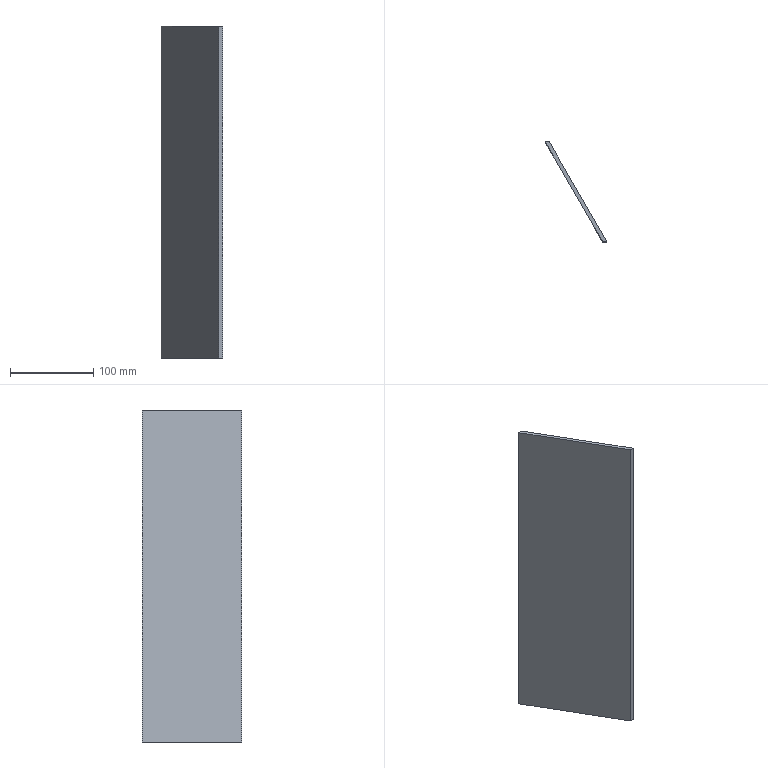Part | SolidWorks | features Extrusion 1 | 1 solid | 6 faces | box 74.282 x 120 x 400 mm | volume 240000 mm3 | plane 6
STEP:
#1=CARTESIAN_POINT('',(0.,0.,0.));
#2=VERTEX_POINT('',#1);
#3=CARTESIAN_POINT('',(69.282,-120.,0.));
#4=VERTEX_POINT('',#3);
#5=CARTESIAN_POINT('',(69.282,-120.,0.));
#6=DIRECTION('',(0.5,-0.866,0.));
#7=VECTOR('',#6,1000.);
#8=LINE('',#5,#7);
#9=EDGE_CURVE('',#2,#4,#8,.T.);
#10=ORIENTED_EDGE('',*,*,#9,.T.);
#11=CARTESIAN_POINT('',(69.282,-120.,400.));
#12=VERTEX_POINT('',#11);
#13=CARTESIAN_POINT('',(69.282,-120.,400.));
#14=DIRECTION('',(0.,0.,-1.));
#15=VECTOR('',#14,1000.);
#16=LINE('',#13,#15);
#17=EDGE_CURVE('',#12,#4,#16,.T.);
#18=ORIENTED_EDGE('',*,*,#17,.F.);
#19=CARTESIAN_POINT('',(0.,0.,400.));
#20=VERTEX_POINT('',#19);
#21=CARTESIAN_POINT('',(69.282,-120.,400.));
#22=DIRECTION('',(0.5,-0.866,0.));
#23=VECTOR('',#22,1000.);
#24=LINE('',#21,#23);
#25=EDGE_CURVE('',#20,#12,#24,.T.);
#26=ORIENTED_EDGE('',*,*,#25,.F.);
#27=CARTESIAN_POINT('',(0.,0.,400.));
#28=DIRECTION('',(0.,0.,-1.));
#29=VECTOR('',#28,1000.);
#30=LINE('',#27,#29);
#31=EDGE_CURVE('',#20,#2,#30,.T.);
#32=ORIENTED_EDGE('',*,*,#31,.T.);
#33=EDGE_LOOP('',(#10,#18,#26,#32));
#34=FACE_OUTER_BOUND('',#33,.T.);
#35=CARTESIAN_POINT('',(69.282,-120.,400.));
#36=DIRECTION('',(0.866,0.5,0.));
#37=DIRECTION('',(-0.5,0.866,0.));
#38=AXIS2_PLACEMENT_3D('',#35,#36,#37);
#39=PLANE('',#38);
#40=ADVANCED_FACE('',(#34),#39,.F.);
#41=CARTESIAN_POINT('',(74.282,-120.,0.));
#42=VERTEX_POINT('',#41);
#43=CARTESIAN_POINT('',(74.282,-120.,0.));
#44=DIRECTION('',(1.,0.,0.));
#45=VECTOR('',#44,1000.);
#46=LINE('',#43,#45);
#47=EDGE_CURVE('',#4,#42,#46,.T.);
#48=ORIENTED_EDGE('',*,*,#47,.T.);
#49=CARTESIAN_POINT('',(74.282,-120.,400.));
#50=VERTEX_POINT('',#49);
#51=CARTESIAN_POINT('',(74.282,-120.,400.));
#52=DIRECTION('',(0.,0.,-1.));
#53=VECTOR('',#52,1000.);
#54=LINE('',#51,#53);
#55=EDGE_CURVE('',#50,#42,#54,.T.);
#56=ORIENTED_EDGE('',*,*,#55,.F.);
#57=CARTESIAN_POINT('',(74.282,-120.,400.));
#58=DIRECTION('',(1.,0.,0.));
#59=VECTOR('',#58,1000.);
#60=LINE('',#57,#59);
#61=EDGE_CURVE('',#12,#50,#60,.T.);
#62=ORIENTED_EDGE('',*,*,#61,.F.);
#63=ORIENTED_EDGE('',*,*,#17,.T.);
#64=EDGE_LOOP('',(#48,#56,#62,#63));
#65=FACE_OUTER_BOUND('',#64,.T.);
#66=CARTESIAN_POINT('',(74.282,-120.,400.));
#67=DIRECTION('',(0.,1.,0.));
#68=DIRECTION('',(0.,0.,1.));
#69=AXIS2_PLACEMENT_3D('',#66,#67,#68);
#70=PLANE('',#69);
#71=ADVANCED_FACE('',(#65),#70,.F.);
#72=CARTESIAN_POINT('',(5.,0.,0.));
#73=VERTEX_POINT('',#72);
#74=CARTESIAN_POINT('',(5.,0.,0.));
#75=DIRECTION('',(-0.5,0.866,0.));
#76=VECTOR('',#75,1000.);
#77=LINE('',#74,#76);
#78=EDGE_CURVE('',#42,#73,#77,.T.);
#79=ORIENTED_EDGE('',*,*,#78,.T.);
#80=CARTESIAN_POINT('',(5.,0.,400.));
#81=VERTEX_POINT('',#80);
#82=CARTESIAN_POINT('',(5.,0.,400.));
#83=DIRECTION('',(0.,0.,-1.));
#84=VECTOR('',#83,1000.);
#85=LINE('',#82,#84);
#86=EDGE_CURVE('',#81,#73,#85,.T.);
#87=ORIENTED_EDGE('',*,*,#86,.F.);
#88=CARTESIAN_POINT('',(5.,0.,400.));
#89=DIRECTION('',(-0.5,0.866,0.));
#90=VECTOR('',#89,1000.);
#91=LINE('',#88,#90);
#92=EDGE_CURVE('',#50,#81,#91,.T.);
#93=ORIENTED_EDGE('',*,*,#92,.F.);
#94=ORIENTED_EDGE('',*,*,#55,.T.);
#95=EDGE_LOOP('',(#79,#87,#93,#94));
#96=FACE_OUTER_BOUND('',#95,.T.);
#97=CARTESIAN_POINT('',(5.,0.,400.));
#98=DIRECTION('',(-0.866,-0.5,0.));
#99=DIRECTION('',(0.5,-0.866,0.));
#100=AXIS2_PLACEMENT_3D('',#97,#98,#99);
#101=PLANE('',#100);
#102=ADVANCED_FACE('',(#96),#101,.F.);
#103=CARTESIAN_POINT('',(0.,0.,0.));
#104=DIRECTION('',(-1.,0.,0.));
#105=VECTOR('',#104,1000.);
#106=LINE('',#103,#105);
#107=EDGE_CURVE('',#73,#2,#106,.T.);
#108=ORIENTED_EDGE('',*,*,#107,.T.);
#109=ORIENTED_EDGE('',*,*,#31,.F.);
#110=CARTESIAN_POINT('',(0.,0.,400.));
#111=DIRECTION('',(-1.,0.,0.));
#112=VECTOR('',#111,1000.);
#113=LINE('',#110,#112);
#114=EDGE_CURVE('',#81,#20,#113,.T.);
#115=ORIENTED_EDGE('',*,*,#114,.F.);
#116=ORIENTED_EDGE('',*,*,#86,.T.);
#117=EDGE_LOOP('',(#108,#109,#115,#116));
#118=FACE_OUTER_BOUND('',#117,.T.);
#119=CARTESIAN_POINT('',(0.,0.,400.));
#120=DIRECTION('',(0.,-1.,0.));
#121=DIRECTION('',(1.,0.,0.));
#122=AXIS2_PLACEMENT_3D('',#119,#120,#121);
#123=PLANE('',#122);
#124=ADVANCED_FACE('',(#118),#123,.F.);
#125=ORIENTED_EDGE('',*,*,#25,.T.);
#126=ORIENTED_EDGE('',*,*,#61,.T.);
#127=ORIENTED_EDGE('',*,*,#92,.T.);
#128=ORIENTED_EDGE('',*,*,#114,.T.);
#129=EDGE_LOOP('',(#125,#126,#127,#128));
#130=FACE_OUTER_BOUND('',#129,.T.);
#131=CARTESIAN_POINT('',(0.,0.,400.));
#132=DIRECTION('',(0.,0.,-1.));
#133=DIRECTION('',(-1.,0.,0.));
#134=AXIS2_PLACEMENT_3D('',#131,#132,#133);
#135=PLANE('',#134);
#136=ADVANCED_FACE('',(#130),#135,.F.);
#137=ORIENTED_EDGE('',*,*,#9,.F.);
#138=ORIENTED_EDGE('',*,*,#107,.F.);
#139=ORIENTED_EDGE('',*,*,#78,.F.);
#140=ORIENTED_EDGE('',*,*,#47,.F.);
#141=EDGE_LOOP('',(#137,#138,#139,#140));
#142=FACE_OUTER_BOUND('',#141,.T.);
#143=CARTESIAN_POINT('',(0.,0.,0.));
#144=DIRECTION('',(0.,0.,-1.));
#145=DIRECTION('',(-1.,0.,0.));
#146=AXIS2_PLACEMENT_3D('',#143,#144,#145);
#147=PLANE('',#146);
#148=ADVANCED_FACE('',(#142),#147,.T.);
#149=CLOSED_SHELL('',(#40,#71,#102,#124,#136,#148));
#150=MANIFOLD_SOLID_BREP('',#149);
#151=CARTESIAN_POINT('',(0.,0.,0.));
#152=DIRECTION('',(0.,0.,1.));
#153=DIRECTION('',(1.,0.,0.));
#154=AXIS2_PLACEMENT_3D('',#151,#152,#153);
#155=(LENGTH_UNIT()NAMED_UNIT(*)SI_UNIT(.MILLI.,.METRE.));
#156=UNCERTAINTY_MEASURE_WITH_UNIT(LENGTH_MEASURE(0.00001),#155,'','');
#157=(NAMED_UNIT(*)PLANE_ANGLE_UNIT()SI_UNIT($,.RADIAN.));
#158=(NAMED_UNIT(*)SI_UNIT($,.STERADIAN.)SOLID_ANGLE_UNIT());
#159=(GEOMETRIC_REPRESENTATION_CONTEXT(3)GLOBAL_UNCERTAINTY_ASSIGNED_CONTEXT((#156))GLOBAL_UNIT_ASSIGNED_CONTEXT((#155,#157,#158))REPRESENTATION_CONTEXT('',''));
#160=ADVANCED_BREP_SHAPE_REPRESENTATION('',(#150,#154),#159);